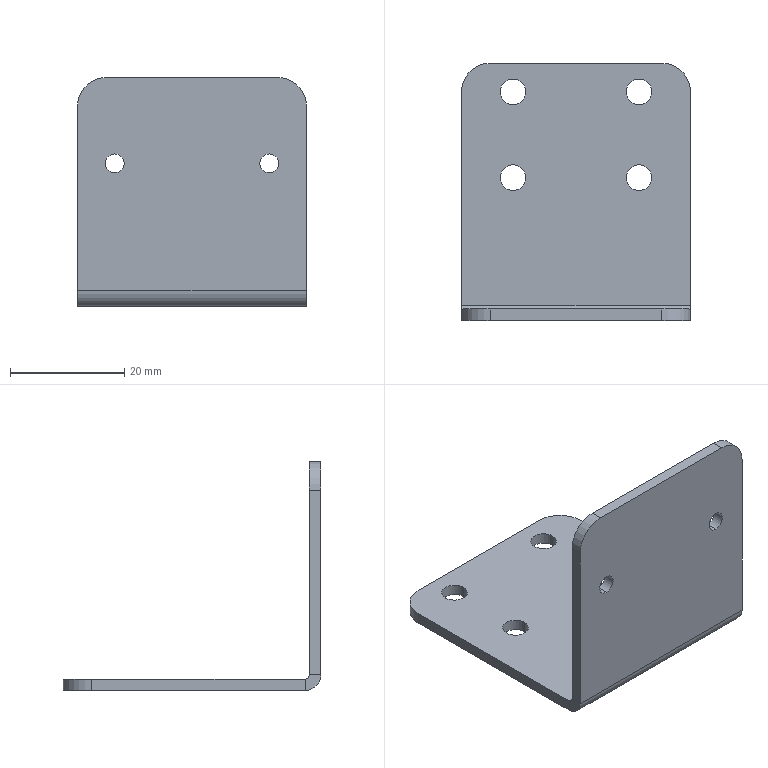Part | STEP file | 1 solid | 30 faces | box 40 x 45 x 40 mm | volume 6376 mm3 | cylinder 18 | plane 12 | commonest cylinder face diameters 4.5 x8 3.3 x4 10 x4 1.473 x1 5.473 x1